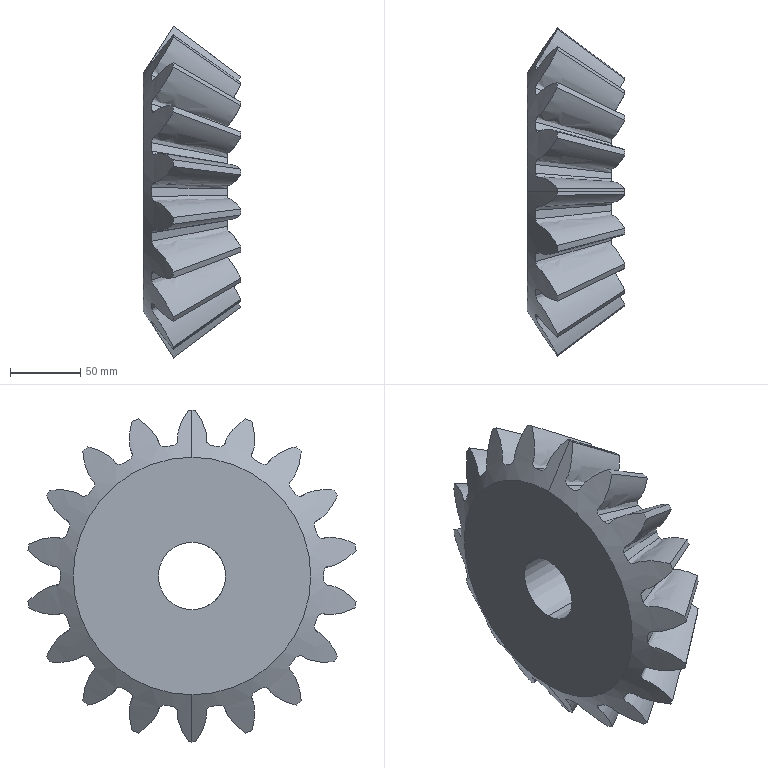Part | SolidWorks | features 3DProfileFeature 12, BlendCut 1, CirPattern 1, ICE 1, RefAxis 1, Revolution 1 | 1 solid | 102 faces | box 69.675 x 233.385 x 236.188 mm | volume 1498219 mm3 | cone 40 | spline 36 | plane 24 | cylinder 2 | commonest cylinder face diameters 47.944 x2